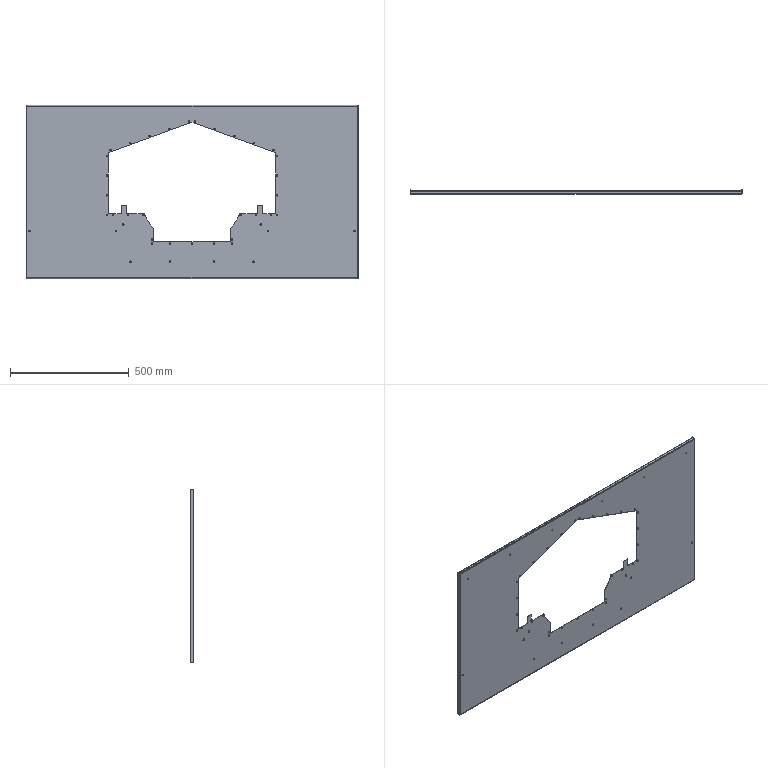Part | NX | features solid 2 | 1 solid | 169 faces | box 1400 x 16 x 730 mm | volume 1232588 mm3 | cylinder 106 | plane 63 | commonest cylinder face diameters 7 x82 6 x17 3 x5 435 x2